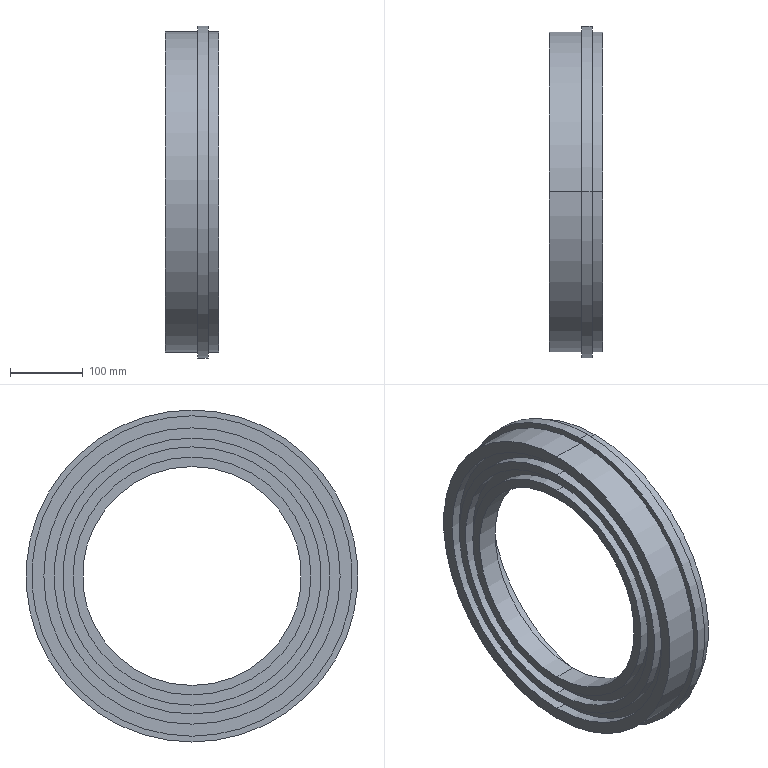Part | SolidWorks | features Revolution 1 | 1 solid | 27 faces | box 74 x 455 x 455 mm | volume 3257613 mm3 | cylinder 18 | plane 9 | commonest cylinder face diameters 439 x4 300 x2 326 x2 354 x2 378 x2 400 x2
STEP:
#1=CARTESIAN_POINT('',(74.,0.,-200.));
#2=VERTEX_POINT('',#1);
#3=CARTESIAN_POINT('',(74.,0.,200.));
#4=VERTEX_POINT('',#3);
#5=CARTESIAN_POINT('',(74.,0.,0.));
#6=DIRECTION('',(-1.,0.,0.));
#7=DIRECTION('',(0.,0.,1.));
#8=AXIS2_PLACEMENT_3D('',#5,#6,#7);
#9=CIRCLE('',#8,200.);
#10=EDGE_CURVE('',#2,#4,#9,.T.);
#11=ORIENTED_EDGE('',*,*,#10,.F.);
#12=CARTESIAN_POINT('',(30.,0.,-200.));
#13=VERTEX_POINT('',#12);
#14=CARTESIAN_POINT('',(0.,0.,-200.));
#15=DIRECTION('',(-1.,0.,0.));
#16=VECTOR('',#15,1000.);
#17=LINE('',#14,#16);
#18=EDGE_CURVE('',#2,#13,#17,.T.);
#19=ORIENTED_EDGE('',*,*,#18,.T.);
#20=CARTESIAN_POINT('',(30.,0.,200.));
#21=VERTEX_POINT('',#20);
#22=CARTESIAN_POINT('',(30.,0.,0.));
#23=DIRECTION('',(-1.,0.,0.));
#24=DIRECTION('',(0.,0.,1.));
#25=AXIS2_PLACEMENT_3D('',#22,#23,#24);
#26=CIRCLE('',#25,200.);
#27=EDGE_CURVE('',#13,#21,#26,.T.);
#28=ORIENTED_EDGE('',*,*,#27,.T.);
#29=CARTESIAN_POINT('',(0.,0.,200.));
#30=DIRECTION('',(-1.,0.,0.));
#31=VECTOR('',#30,1000.);
#32=LINE('',#29,#31);
#33=EDGE_CURVE('',#4,#21,#32,.T.);
#34=ORIENTED_EDGE('',*,*,#33,.F.);
#35=EDGE_LOOP('',(#11,#19,#28,#34));
#36=FACE_OUTER_BOUND('',#35,.T.);
#37=CARTESIAN_POINT('',(0.,0.,0.));
#38=DIRECTION('',(-1.,0.,0.));
#39=DIRECTION('',(0.,0.,1.));
#40=AXIS2_PLACEMENT_3D('',#37,#38,#39);
#41=CYLINDRICAL_SURFACE('',#40,200.);
#42=ADVANCED_FACE('',(#36),#41,.F.);
#43=CARTESIAN_POINT('',(74.,0.,219.5));
#44=VERTEX_POINT('',#43);
#45=CARTESIAN_POINT('',(74.,0.,-219.5));
#46=VERTEX_POINT('',#45);
#47=CARTESIAN_POINT('',(74.,0.,0.));
#48=DIRECTION('',(-1.,0.,0.));
#49=DIRECTION('',(0.,0.,1.));
#50=AXIS2_PLACEMENT_3D('',#47,#48,#49);
#51=CIRCLE('',#50,219.5);
#52=EDGE_CURVE('',#44,#46,#51,.T.);
#53=ORIENTED_EDGE('',*,*,#52,.T.);
#54=CARTESIAN_POINT('',(59.,0.,-219.5));
#55=VERTEX_POINT('',#54);
#56=CARTESIAN_POINT('',(0.,0.,-219.5));
#57=DIRECTION('',(-1.,0.,0.));
#58=VECTOR('',#57,1000.);
#59=LINE('',#56,#58);
#60=EDGE_CURVE('',#46,#55,#59,.T.);
#61=ORIENTED_EDGE('',*,*,#60,.T.);
#62=CARTESIAN_POINT('',(59.,0.,219.5));
#63=VERTEX_POINT('',#62);
#64=CARTESIAN_POINT('',(59.,0.,0.));
#65=DIRECTION('',(-1.,0.,0.));
#66=DIRECTION('',(0.,0.,1.));
#67=AXIS2_PLACEMENT_3D('',#64,#65,#66);
#68=CIRCLE('',#67,219.5);
#69=EDGE_CURVE('',#63,#55,#68,.T.);
#70=ORIENTED_EDGE('',*,*,#69,.F.);
#71=CARTESIAN_POINT('',(0.,0.,219.5));
#72=DIRECTION('',(-1.,0.,0.));
#73=VECTOR('',#72,1000.);
#74=LINE('',#71,#73);
#75=EDGE_CURVE('',#44,#63,#74,.T.);
#76=ORIENTED_EDGE('',*,*,#75,.F.);
#77=EDGE_LOOP('',(#53,#61,#70,#76));
#78=FACE_OUTER_BOUND('',#77,.T.);
#79=CARTESIAN_POINT('',(0.,0.,0.));
#80=DIRECTION('',(-1.,0.,0.));
#81=DIRECTION('',(0.,0.,1.));
#82=AXIS2_PLACEMENT_3D('',#79,#80,#81);
#83=CYLINDRICAL_SURFACE('',#82,219.5);
#84=ADVANCED_FACE('',(#78),#83,.T.);
#85=CARTESIAN_POINT('',(59.,0.,227.5));
#86=VERTEX_POINT('',#85);
#87=CARTESIAN_POINT('',(59.,0.,-227.5));
#88=VERTEX_POINT('',#87);
#89=CARTESIAN_POINT('',(59.,0.,0.));
#90=DIRECTION('',(-1.,0.,0.));
#91=DIRECTION('',(0.,0.,1.));
#92=AXIS2_PLACEMENT_3D('',#89,#90,#91);
#93=CIRCLE('',#92,227.5);
#94=EDGE_CURVE('',#86,#88,#93,.T.);
#95=ORIENTED_EDGE('',*,*,#94,.T.);
#96=CARTESIAN_POINT('',(45.,0.,-227.5));
#97=VERTEX_POINT('',#96);
#98=CARTESIAN_POINT('',(0.,0.,-227.5));
#99=DIRECTION('',(-1.,0.,0.));
#100=VECTOR('',#99,1000.);
#101=LINE('',#98,#100);
#102=EDGE_CURVE('',#88,#97,#101,.T.);
#103=ORIENTED_EDGE('',*,*,#102,.T.);
#104=CARTESIAN_POINT('',(45.,0.,227.5));
#105=VERTEX_POINT('',#104);
#106=CARTESIAN_POINT('',(45.,0.,0.));
#107=DIRECTION('',(-1.,0.,0.));
#108=DIRECTION('',(0.,0.,1.));
#109=AXIS2_PLACEMENT_3D('',#106,#107,#108);
#110=CIRCLE('',#109,227.5);
#111=EDGE_CURVE('',#105,#97,#110,.T.);
#112=ORIENTED_EDGE('',*,*,#111,.F.);
#113=CARTESIAN_POINT('',(0.,0.,227.5));
#114=DIRECTION('',(-1.,0.,0.));
#115=VECTOR('',#114,1000.);
#116=LINE('',#113,#115);
#117=EDGE_CURVE('',#86,#105,#116,.T.);
#118=ORIENTED_EDGE('',*,*,#117,.F.);
#119=EDGE_LOOP('',(#95,#103,#112,#118));
#120=FACE_OUTER_BOUND('',#119,.T.);
#121=CARTESIAN_POINT('',(0.,0.,0.));
#122=DIRECTION('',(-1.,0.,0.));
#123=DIRECTION('',(0.,0.,1.));
#124=AXIS2_PLACEMENT_3D('',#121,#122,#123);
#125=CYLINDRICAL_SURFACE('',#124,227.5);
#126=ADVANCED_FACE('',(#120),#125,.T.);
#127=CARTESIAN_POINT('',(45.,0.,219.5));
#128=VERTEX_POINT('',#127);
#129=CARTESIAN_POINT('',(45.,0.,-219.5));
#130=VERTEX_POINT('',#129);
#131=CARTESIAN_POINT('',(45.,0.,0.));
#132=DIRECTION('',(-1.,0.,0.));
#133=DIRECTION('',(0.,0.,1.));
#134=AXIS2_PLACEMENT_3D('',#131,#132,#133);
#135=CIRCLE('',#134,219.5);
#136=EDGE_CURVE('',#128,#130,#135,.T.);
#137=ORIENTED_EDGE('',*,*,#136,.T.);
#138=CARTESIAN_POINT('',(0.,0.,-219.5));
#139=VERTEX_POINT('',#138);
#140=CARTESIAN_POINT('',(0.,0.,-219.5));
#141=DIRECTION('',(-1.,0.,0.));
#142=VECTOR('',#141,1000.);
#143=LINE('',#140,#142);
#144=EDGE_CURVE('',#130,#139,#143,.T.);
#145=ORIENTED_EDGE('',*,*,#144,.T.);
#146=CARTESIAN_POINT('',(0.,0.,219.5));
#147=VERTEX_POINT('',#146);
#148=CARTESIAN_POINT('',(0.,0.,0.));
#149=DIRECTION('',(-1.,0.,0.));
#150=DIRECTION('',(0.,0.,1.));
#151=AXIS2_PLACEMENT_3D('',#148,#149,#150);
#152=CIRCLE('',#151,219.5);
#153=EDGE_CURVE('',#147,#139,#152,.T.);
#154=ORIENTED_EDGE('',*,*,#153,.F.);
#155=CARTESIAN_POINT('',(0.,0.,219.5));
#156=DIRECTION('',(-1.,0.,0.));
#157=VECTOR('',#156,1000.);
#158=LINE('',#155,#157);
#159=EDGE_CURVE('',#128,#147,#158,.T.);
#160=ORIENTED_EDGE('',*,*,#159,.F.);
#161=EDGE_LOOP('',(#137,#145,#154,#160));
#162=FACE_OUTER_BOUND('',#161,.T.);
#163=CARTESIAN_POINT('',(0.,0.,0.));
#164=DIRECTION('',(-1.,0.,0.));
#165=DIRECTION('',(0.,0.,1.));
#166=AXIS2_PLACEMENT_3D('',#163,#164,#165);
#167=CYLINDRICAL_SURFACE('',#166,219.5);
#168=ADVANCED_FACE('',(#162),#167,.T.);
#169=CARTESIAN_POINT('',(14.,0.,-203.));
#170=VERTEX_POINT('',#169);
#171=CARTESIAN_POINT('',(14.,0.,203.));
#172=VERTEX_POINT('',#171);
#173=CARTESIAN_POINT('',(14.,0.,0.));
#174=DIRECTION('',(-1.,0.,0.));
#175=DIRECTION('',(0.,0.,1.));
#176=AXIS2_PLACEMENT_3D('',#173,#174,#175);
#177=CIRCLE('',#176,203.);
#178=EDGE_CURVE('',#170,#172,#177,.T.);
#179=ORIENTED_EDGE('',*,*,#178,.F.);
#180=CARTESIAN_POINT('',(0.,0.,-203.));
#181=VERTEX_POINT('',#180);
#182=CARTESIAN_POINT('',(0.,0.,-203.));
#183=DIRECTION('',(-1.,0.,0.));
#184=VECTOR('',#183,1000.);
#185=LINE('',#182,#184);
#186=EDGE_CURVE('',#170,#181,#185,.T.);
#187=ORIENTED_EDGE('',*,*,#186,.T.);
#188=CARTESIAN_POINT('',(0.,0.,203.));
#189=VERTEX_POINT('',#188);
#190=CARTESIAN_POINT('',(0.,0.,0.));
#191=DIRECTION('',(-1.,0.,0.));
#192=DIRECTION('',(0.,0.,1.));
#193=AXIS2_PLACEMENT_3D('',#190,#191,#192);
#194=CIRCLE('',#193,203.);
#195=EDGE_CURVE('',#181,#189,#194,.T.);
#196=ORIENTED_EDGE('',*,*,#195,.T.);
#197=CARTESIAN_POINT('',(0.,0.,203.));
#198=DIRECTION('',(-1.,0.,0.));
#199=VECTOR('',#198,1000.);
#200=LINE('',#197,#199);
#201=EDGE_CURVE('',#172,#189,#200,.T.);
#202=ORIENTED_EDGE('',*,*,#201,.F.);
#203=EDGE_LOOP('',(#179,#187,#196,#202));
#204=FACE_OUTER_BOUND('',#203,.T.);
#205=CARTESIAN_POINT('',(0.,0.,0.));
#206=DIRECTION('',(-1.,0.,0.));
#207=DIRECTION('',(0.,0.,1.));
#208=AXIS2_PLACEMENT_3D('',#205,#206,#207);
#209=CYLINDRICAL_SURFACE('',#208,203.);
#210=ADVANCED_FACE('',(#204),#209,.F.);
#211=CARTESIAN_POINT('',(14.,0.,189.));
#212=VERTEX_POINT('',#211);
#213=CARTESIAN_POINT('',(14.,0.,-189.));
#214=VERTEX_POINT('',#213);
#215=CARTESIAN_POINT('',(14.,0.,0.));
#216=DIRECTION('',(-1.,0.,0.));
#217=DIRECTION('',(0.,0.,1.));
#218=AXIS2_PLACEMENT_3D('',#215,#216,#217);
#219=CIRCLE('',#218,189.);
#220=EDGE_CURVE('',#212,#214,#219,.T.);
#221=ORIENTED_EDGE('',*,*,#220,.T.);
#222=CARTESIAN_POINT('',(0.,0.,-189.));
#223=VERTEX_POINT('',#222);
#224=CARTESIAN_POINT('',(0.,0.,-189.));
#225=DIRECTION('',(-1.,0.,0.));
#226=VECTOR('',#225,1000.);
#227=LINE('',#224,#226);
#228=EDGE_CURVE('',#214,#223,#227,.T.);
#229=ORIENTED_EDGE('',*,*,#228,.T.);
#230=CARTESIAN_POINT('',(0.,0.,189.));
#231=VERTEX_POINT('',#230);
#232=CARTESIAN_POINT('',(0.,0.,0.));
#233=DIRECTION('',(-1.,0.,0.));
#234=DIRECTION('',(0.,0.,1.));
#235=AXIS2_PLACEMENT_3D('',#232,#233,#234);
#236=CIRCLE('',#235,189.);
#237=EDGE_CURVE('',#231,#223,#236,.T.);
#238=ORIENTED_EDGE('',*,*,#237,.F.);
#239=CARTESIAN_POINT('',(0.,0.,189.));
#240=DIRECTION('',(-1.,0.,0.));
#241=VECTOR('',#240,1000.);
#242=LINE('',#239,#241);
#243=EDGE_CURVE('',#212,#231,#242,.T.);
#244=ORIENTED_EDGE('',*,*,#243,.F.);
#245=EDGE_LOOP('',(#221,#229,#238,#244));
#246=FACE_OUTER_BOUND('',#245,.T.);
#247=CARTESIAN_POINT('',(0.,0.,0.));
#248=DIRECTION('',(-1.,0.,0.));
#249=DIRECTION('',(0.,0.,1.));
#250=AXIS2_PLACEMENT_3D('',#247,#248,#249);
#251=CYLINDRICAL_SURFACE('',#250,189.);
#252=ADVANCED_FACE('',(#246),#251,.T.);
#253=CARTESIAN_POINT('',(14.,0.,-177.));
#254=VERTEX_POINT('',#253);
#255=CARTESIAN_POINT('',(14.,0.,177.));
#256=VERTEX_POINT('',#255);
#257=CARTESIAN_POINT('',(14.,0.,0.));
#258=DIRECTION('',(-1.,0.,0.));
#259=DIRECTION('',(0.,0.,1.));
#260=AXIS2_PLACEMENT_3D('',#257,#258,#259);
#261=CIRCLE('',#260,177.);
#262=EDGE_CURVE('',#254,#256,#261,.T.);
#263=ORIENTED_EDGE('',*,*,#262,.F.);
#264=CARTESIAN_POINT('',(0.,0.,-177.));
#265=VERTEX_POINT('',#264);
#266=CARTESIAN_POINT('',(0.,0.,-177.));
#267=DIRECTION('',(-1.,0.,0.));
#268=VECTOR('',#267,1000.);
#269=LINE('',#266,#268);
#270=EDGE_CURVE('',#254,#265,#269,.T.);
#271=ORIENTED_EDGE('',*,*,#270,.T.);
#272=CARTESIAN_POINT('',(0.,0.,177.));
#273=VERTEX_POINT('',#272);
#274=CARTESIAN_POINT('',(0.,0.,0.));
#275=DIRECTION('',(-1.,0.,0.));
#276=DIRECTION('',(0.,0.,1.));
#277=AXIS2_PLACEMENT_3D('',#274,#275,#276);
#278=CIRCLE('',#277,177.);
#279=EDGE_CURVE('',#265,#273,#278,.T.);
#280=ORIENTED_EDGE('',*,*,#279,.T.);
#281=CARTESIAN_POINT('',(0.,0.,177.));
#282=DIRECTION('',(-1.,0.,0.));
#283=VECTOR('',#282,1000.);
#284=LINE('',#281,#283);
#285=EDGE_CURVE('',#256,#273,#284,.T.);
#286=ORIENTED_EDGE('',*,*,#285,.F.);
#287=EDGE_LOOP('',(#263,#271,#280,#286));
#288=FACE_OUTER_BOUND('',#287,.T.);
#289=CARTESIAN_POINT('',(0.,0.,0.));
#290=DIRECTION('',(-1.,0.,0.));
#291=DIRECTION('',(0.,0.,1.));
#292=AXIS2_PLACEMENT_3D('',#289,#290,#291);
#293=CYLINDRICAL_SURFACE('',#292,177.);
#294=ADVANCED_FACE('',(#288),#293,.F.);
#295=CARTESIAN_POINT('',(14.,0.,163.));
#296=VERTEX_POINT('',#295);
#297=CARTESIAN_POINT('',(14.,0.,-163.));
#298=VERTEX_POINT('',#297);
#299=CARTESIAN_POINT('',(14.,0.,0.));
#300=DIRECTION('',(-1.,0.,0.));
#301=DIRECTION('',(0.,0.,1.));
#302=AXIS2_PLACEMENT_3D('',#299,#300,#301);
#303=CIRCLE('',#302,163.);
#304=EDGE_CURVE('',#296,#298,#303,.T.);
#305=ORIENTED_EDGE('',*,*,#304,.T.);
#306=CARTESIAN_POINT('',(0.,0.,-163.));
#307=VERTEX_POINT('',#306);
#308=CARTESIAN_POINT('',(0.,0.,-163.));
#309=DIRECTION('',(-1.,0.,0.));
#310=VECTOR('',#309,1000.);
#311=LINE('',#308,#310);
#312=EDGE_CURVE('',#298,#307,#311,.T.);
#313=ORIENTED_EDGE('',*,*,#312,.T.);
#314=CARTESIAN_POINT('',(0.,0.,163.));
#315=VERTEX_POINT('',#314);
#316=CARTESIAN_POINT('',(0.,0.,0.));
#317=DIRECTION('',(-1.,0.,0.));
#318=DIRECTION('',(0.,0.,1.));
#319=AXIS2_PLACEMENT_3D('',#316,#317,#318);
#320=CIRCLE('',#319,163.);
#321=EDGE_CURVE('',#315,#307,#320,.T.);
#322=ORIENTED_EDGE('',*,*,#321,.F.);
#323=CARTESIAN_POINT('',(0.,0.,163.));
#324=DIRECTION('',(-1.,0.,0.));
#325=VECTOR('',#324,1000.);
#326=LINE('',#323,#325);
#327=EDGE_CURVE('',#296,#315,#326,.T.);
#328=ORIENTED_EDGE('',*,*,#327,.F.);
#329=EDGE_LOOP('',(#305,#313,#322,#328));
#330=FACE_OUTER_BOUND('',#329,.T.);
#331=CARTESIAN_POINT('',(0.,0.,0.));
#332=DIRECTION('',(-1.,0.,0.));
#333=DIRECTION('',(0.,0.,1.));
#334=AXIS2_PLACEMENT_3D('',#331,#332,#333);
#335=CYLINDRICAL_SURFACE('',#334,163.);
#336=ADVANCED_FACE('',(#330),#335,.T.);
#337=CARTESIAN_POINT('',(30.,0.,-150.));
#338=VERTEX_POINT('',#337);
#339=CARTESIAN_POINT('',(30.,0.,150.));
#340=VERTEX_POINT('',#339);
#341=CARTESIAN_POINT('',(30.,0.,0.));
#342=DIRECTION('',(-1.,0.,0.));
#343=DIRECTION('',(0.,0.,1.));
#344=AXIS2_PLACEMENT_3D('',#341,#342,#343);
#345=CIRCLE('',#344,150.);
#346=EDGE_CURVE('',#338,#340,#345,.T.);
#347=ORIENTED_EDGE('',*,*,#346,.F.);
#348=CARTESIAN_POINT('',(0.,0.,-150.));
#349=VERTEX_POINT('',#348);
#350=CARTESIAN_POINT('',(0.,0.,-150.));
#351=DIRECTION('',(-1.,0.,0.));
#352=VECTOR('',#351,1000.);
#353=LINE('',#350,#352);
#354=EDGE_CURVE('',#338,#349,#353,.T.);
#355=ORIENTED_EDGE('',*,*,#354,.T.);
#356=CARTESIAN_POINT('',(0.,0.,150.));
#357=VERTEX_POINT('',#356);
#358=CARTESIAN_POINT('',(0.,0.,0.));
#359=DIRECTION('',(-1.,0.,0.));
#360=DIRECTION('',(0.,0.,1.));
#361=AXIS2_PLACEMENT_3D('',#358,#359,#360);
#362=CIRCLE('',#361,150.);
#363=EDGE_CURVE('',#349,#357,#362,.T.);
#364=ORIENTED_EDGE('',*,*,#363,.T.);
#365=CARTESIAN_POINT('',(0.,0.,150.));
#366=DIRECTION('',(-1.,0.,0.));
#367=VECTOR('',#366,1000.);
#368=LINE('',#365,#367);
#369=EDGE_CURVE('',#340,#357,#368,.T.);
#370=ORIENTED_EDGE('',*,*,#369,.F.);
#371=EDGE_LOOP('',(#347,#355,#364,#370));
#372=FACE_OUTER_BOUND('',#371,.T.);
#373=CARTESIAN_POINT('',(0.,0.,0.));
#374=DIRECTION('',(-1.,0.,0.));
#375=DIRECTION('',(0.,0.,1.));
#376=AXIS2_PLACEMENT_3D('',#373,#374,#375);
#377=CYLINDRICAL_SURFACE('',#376,150.);
#378=ADVANCED_FACE('',(#372),#377,.F.);
#379=ORIENTED_EDGE('',*,*,#354,.F.);
#380=CARTESIAN_POINT('',(30.,0.,0.));
#381=DIRECTION('',(-1.,0.,0.));
#382=DIRECTION('',(0.,0.,1.));
#383=AXIS2_PLACEMENT_3D('',#380,#381,#382);
#384=CIRCLE('',#383,150.);
#385=EDGE_CURVE('',#340,#338,#384,.T.);
#386=ORIENTED_EDGE('',*,*,#385,.F.);
#387=ORIENTED_EDGE('',*,*,#369,.T.);
#388=CARTESIAN_POINT('',(0.,0.,0.));
#389=DIRECTION('',(-1.,0.,0.));
#390=DIRECTION('',(0.,0.,1.));
#391=AXIS2_PLACEMENT_3D('',#388,#389,#390);
#392=CIRCLE('',#391,150.);
#393=EDGE_CURVE('',#357,#349,#392,.T.);
#394=ORIENTED_EDGE('',*,*,#393,.T.);
#395=EDGE_LOOP('',(#379,#386,#387,#394));
#396=FACE_OUTER_BOUND('',#395,.T.);
#397=CARTESIAN_POINT('',(0.,0.,0.));
#398=DIRECTION('',(-1.,0.,0.));
#399=DIRECTION('',(0.,0.,1.));
#400=AXIS2_PLACEMENT_3D('',#397,#398,#399);
#401=CYLINDRICAL_SURFACE('',#400,150.);
#402=ADVANCED_FACE('',(#396),#401,.F.);
#403=ORIENTED_EDGE('',*,*,#393,.F.);
#404=ORIENTED_EDGE('',*,*,#363,.F.);
#405=EDGE_LOOP('',(#403,#404));
#406=FACE_BOUND('',#405,.T.);
#407=ORIENTED_EDGE('',*,*,#321,.T.);
#408=CARTESIAN_POINT('',(0.,0.,0.));
#409=DIRECTION('',(-1.,0.,0.));
#410=DIRECTION('',(0.,0.,1.));
#411=AXIS2_PLACEMENT_3D('',#408,#409,#410);
#412=CIRCLE('',#411,163.);
#413=EDGE_CURVE('',#307,#315,#412,.T.);
#414=ORIENTED_EDGE('',*,*,#413,.T.);
#415=EDGE_LOOP('',(#407,#414));
#416=FACE_OUTER_BOUND('',#415,.T.);
#417=CARTESIAN_POINT('',(0.,0.,-150.));
#418=DIRECTION('',(1.,0.,0.));
#419=DIRECTION('',(0.,0.,-1.));
#420=AXIS2_PLACEMENT_3D('',#417,#418,#419);
#421=PLANE('',#420);
#422=ADVANCED_FACE('',(#406,#416),#421,.F.);
#423=ORIENTED_EDGE('',*,*,#312,.F.);
#424=CARTESIAN_POINT('',(14.,0.,0.));
#425=DIRECTION('',(-1.,0.,0.));
#426=DIRECTION('',(0.,0.,1.));
#427=AXIS2_PLACEMENT_3D('',#424,#425,#426);
#428=CIRCLE('',#427,163.);
#429=EDGE_CURVE('',#298,#296,#428,.T.);
#430=ORIENTED_EDGE('',*,*,#429,.T.);
#431=ORIENTED_EDGE('',*,*,#327,.T.);
#432=ORIENTED_EDGE('',*,*,#413,.F.);
#433=EDGE_LOOP('',(#423,#430,#431,#432));
#434=FACE_OUTER_BOUND('',#433,.T.);
#435=CARTESIAN_POINT('',(0.,0.,0.));
#436=DIRECTION('',(-1.,0.,0.));
#437=DIRECTION('',(0.,0.,1.));
#438=AXIS2_PLACEMENT_3D('',#435,#436,#437);
#439=CYLINDRICAL_SURFACE('',#438,163.);
#440=ADVANCED_FACE('',(#434),#439,.T.);
#441=ORIENTED_EDGE('',*,*,#304,.F.);
#442=ORIENTED_EDGE('',*,*,#429,.F.);
#443=EDGE_LOOP('',(#441,#442));
#444=FACE_BOUND('',#443,.T.);
#445=CARTESIAN_POINT('',(14.,0.,0.));
#446=DIRECTION('',(-1.,0.,0.));
#447=DIRECTION('',(0.,0.,1.));
#448=AXIS2_PLACEMENT_3D('',#445,#446,#447);
#449=CIRCLE('',#448,177.);
#450=EDGE_CURVE('',#256,#254,#449,.T.);
#451=ORIENTED_EDGE('',*,*,#450,.T.);
#452=ORIENTED_EDGE('',*,*,#262,.T.);
#453=EDGE_LOOP('',(#451,#452));
#454=FACE_OUTER_BOUND('',#453,.T.);
#455=CARTESIAN_POINT('',(14.,0.,-177.));
#456=DIRECTION('',(1.,0.,0.));
#457=DIRECTION('',(0.,0.,-1.));
#458=AXIS2_PLACEMENT_3D('',#455,#456,#457);
#459=PLANE('',#458);
#460=ADVANCED_FACE('',(#444,#454),#459,.F.);
#461=ORIENTED_EDGE('',*,*,#270,.F.);
#462=ORIENTED_EDGE('',*,*,#450,.F.);
#463=ORIENTED_EDGE('',*,*,#285,.T.);
#464=CARTESIAN_POINT('',(0.,0.,0.));
#465=DIRECTION('',(-1.,0.,0.));
#466=DIRECTION('',(0.,0.,1.));
#467=AXIS2_PLACEMENT_3D('',#464,#465,#466);
#468=CIRCLE('',#467,177.);
#469=EDGE_CURVE('',#273,#265,#468,.T.);
#470=ORIENTED_EDGE('',*,*,#469,.T.);
#471=EDGE_LOOP('',(#461,#462,#463,#470));
#472=FACE_OUTER_BOUND('',#471,.T.);
#473=CARTESIAN_POINT('',(0.,0.,0.));
#474=DIRECTION('',(-1.,0.,0.));
#475=DIRECTION('',(0.,0.,1.));
#476=AXIS2_PLACEMENT_3D('',#473,#474,#475);
#477=CYLINDRICAL_SURFACE('',#476,177.);
#478=ADVANCED_FACE('',(#472),#477,.F.);
#479=ORIENTED_EDGE('',*,*,#469,.F.);
#480=ORIENTED_EDGE('',*,*,#279,.F.);
#481=EDGE_LOOP('',(#479,#480));
#482=FACE_BOUND('',#481,.T.);
#483=ORIENTED_EDGE('',*,*,#237,.T.);
#484=CARTESIAN_POINT('',(0.,0.,0.));
#485=DIRECTION('',(-1.,0.,0.));
#486=DIRECTION('',(0.,0.,1.));
#487=AXIS2_PLACEMENT_3D('',#484,#485,#486);
#488=CIRCLE('',#487,189.);
#489=EDGE_CURVE('',#223,#231,#488,.T.);
#490=ORIENTED_EDGE('',*,*,#489,.T.);
#491=EDGE_LOOP('',(#483,#490));
#492=FACE_OUTER_BOUND('',#491,.T.);
#493=CARTESIAN_POINT('',(0.,0.,-177.));
#494=DIRECTION('',(1.,0.,0.));
#495=DIRECTION('',(0.,0.,-1.));
#496=AXIS2_PLACEMENT_3D('',#493,#494,#495);
#497=PLANE('',#496);
#498=ADVANCED_FACE('',(#482,#492),#497,.F.);
#499=ORIENTED_EDGE('',*,*,#228,.F.);
#500=CARTESIAN_POINT('',(14.,0.,0.));
#501=DIRECTION('',(-1.,0.,0.));
#502=DIRECTION('',(0.,0.,1.));
#503=AXIS2_PLACEMENT_3D('',#500,#501,#502);
#504=CIRCLE('',#503,189.);
#505=EDGE_CURVE('',#214,#212,#504,.T.);
#506=ORIENTED_EDGE('',*,*,#505,.T.);
#507=ORIENTED_EDGE('',*,*,#243,.T.);
#508=ORIENTED_EDGE('',*,*,#489,.F.);
#509=EDGE_LOOP('',(#499,#506,#507,#508));
#510=FACE_OUTER_BOUND('',#509,.T.);
#511=CARTESIAN_POINT('',(0.,0.,0.));
#512=DIRECTION('',(-1.,0.,0.));
#513=DIRECTION('',(0.,0.,1.));
#514=AXIS2_PLACEMENT_3D('',#511,#512,#513);
#515=CYLINDRICAL_SURFACE('',#514,189.);
#516=ADVANCED_FACE('',(#510),#515,.T.);
#517=ORIENTED_EDGE('',*,*,#220,.F.);
#518=ORIENTED_EDGE('',*,*,#505,.F.);
#519=EDGE_LOOP('',(#517,#518));
#520=FACE_BOUND('',#519,.T.);
#521=CARTESIAN_POINT('',(14.,0.,0.));
#522=DIRECTION('',(-1.,0.,0.));
#523=DIRECTION('',(0.,0.,1.));
#524=AXIS2_PLACEMENT_3D('',#521,#522,#523);
#525=CIRCLE('',#524,203.);
#526=EDGE_CURVE('',#172,#170,#525,.T.);
#527=ORIENTED_EDGE('',*,*,#526,.T.);
#528=ORIENTED_EDGE('',*,*,#178,.T.);
#529=EDGE_LOOP('',(#527,#528));
#530=FACE_OUTER_BOUND('',#529,.T.);
#531=CARTESIAN_POINT('',(14.,0.,-203.));
#532=DIRECTION('',(1.,0.,0.));
#533=DIRECTION('',(0.,0.,-1.));
#534=AXIS2_PLACEMENT_3D('',#531,#532,#533);
#535=PLANE('',#534);
#536=ADVANCED_FACE('',(#520,#530),#535,.F.);
#537=ORIENTED_EDGE('',*,*,#186,.F.);
#538=ORIENTED_EDGE('',*,*,#526,.F.);
#539=ORIENTED_EDGE('',*,*,#201,.T.);
#540=CARTESIAN_POINT('',(0.,0.,0.));
#541=DIRECTION('',(-1.,0.,0.));
#542=DIRECTION('',(0.,0.,1.));
#543=AXIS2_PLACEMENT_3D('',#540,#541,#542);
#544=CIRCLE('',#543,203.);
#545=EDGE_CURVE('',#189,#181,#544,.T.);
#546=ORIENTED_EDGE('',*,*,#545,.T.);
#547=EDGE_LOOP('',(#537,#538,#539,#546));
#548=FACE_OUTER_BOUND('',#547,.T.);
#549=CARTESIAN_POINT('',(0.,0.,0.));
#550=DIRECTION('',(-1.,0.,0.));
#551=DIRECTION('',(0.,0.,1.));
#552=AXIS2_PLACEMENT_3D('',#549,#550,#551);
#553=CYLINDRICAL_SURFACE('',#552,203.);
#554=ADVANCED_FACE('',(#548),#553,.F.);
#555=ORIENTED_EDGE('',*,*,#545,.F.);
#556=ORIENTED_EDGE('',*,*,#195,.F.);
#557=EDGE_LOOP('',(#555,#556));
#558=FACE_BOUND('',#557,.T.);
#559=ORIENTED_EDGE('',*,*,#153,.T.);
#560=CARTESIAN_POINT('',(0.,0.,0.));
#561=DIRECTION('',(-1.,0.,0.));
#562=DIRECTION('',(0.,0.,1.));
#563=AXIS2_PLACEMENT_3D('',#560,#561,#562);
#564=CIRCLE('',#563,219.5);
#565=EDGE_CURVE('',#139,#147,#564,.T.);
#566=ORIENTED_EDGE('',*,*,#565,.T.);
#567=EDGE_LOOP('',(#559,#566));
#568=FACE_OUTER_BOUND('',#567,.T.);
#569=CARTESIAN_POINT('',(0.,0.,-203.));
#570=DIRECTION('',(1.,0.,0.));
#571=DIRECTION('',(0.,0.,-1.));
#572=AXIS2_PLACEMENT_3D('',#569,#570,#571);
#573=PLANE('',#572);
#574=ADVANCED_FACE('',(#558,#568),#573,.F.);
#575=ORIENTED_EDGE('',*,*,#144,.F.);
#576=CARTESIAN_POINT('',(45.,0.,0.));
#577=DIRECTION('',(-1.,0.,0.));
#578=DIRECTION('',(0.,0.,1.));
#579=AXIS2_PLACEMENT_3D('',#576,#577,#578);
#580=CIRCLE('',#579,219.5);
#581=EDGE_CURVE('',#130,#128,#580,.T.);
#582=ORIENTED_EDGE('',*,*,#581,.T.);
#583=ORIENTED_EDGE('',*,*,#159,.T.);
#584=ORIENTED_EDGE('',*,*,#565,.F.);
#585=EDGE_LOOP('',(#575,#582,#583,#584));
#586=FACE_OUTER_BOUND('',#585,.T.);
#587=CARTESIAN_POINT('',(0.,0.,0.));
#588=DIRECTION('',(-1.,0.,0.));
#589=DIRECTION('',(0.,0.,1.));
#590=AXIS2_PLACEMENT_3D('',#587,#588,#589);
#591=CYLINDRICAL_SURFACE('',#590,219.5);
#592=ADVANCED_FACE('',(#586),#591,.T.);
#593=ORIENTED_EDGE('',*,*,#136,.F.);
#594=ORIENTED_EDGE('',*,*,#581,.F.);
#595=EDGE_LOOP('',(#593,#594));
#596=FACE_BOUND('',#595,.T.);
#597=ORIENTED_EDGE('',*,*,#111,.T.);
#598=CARTESIAN_POINT('',(45.,0.,0.));
#599=DIRECTION('',(-1.,0.,0.));
#600=DIRECTION('',(0.,0.,1.));
#601=AXIS2_PLACEMENT_3D('',#598,#599,#600);
#602=CIRCLE('',#601,227.5);
#603=EDGE_CURVE('',#97,#105,#602,.T.);
#604=ORIENTED_EDGE('',*,*,#603,.T.);
#605=EDGE_LOOP('',(#597,#604));
#606=FACE_OUTER_BOUND('',#605,.T.);
#607=CARTESIAN_POINT('',(45.,0.,-219.5));
#608=DIRECTION('',(1.,0.,0.));
#609=DIRECTION('',(0.,0.,-1.));
#610=AXIS2_PLACEMENT_3D('',#607,#608,#609);
#611=PLANE('',#610);
#612=ADVANCED_FACE('',(#596,#606),#611,.F.);
#613=ORIENTED_EDGE('',*,*,#102,.F.);
#614=CARTESIAN_POINT('',(59.,0.,0.));
#615=DIRECTION('',(-1.,0.,0.));
#616=DIRECTION('',(0.,0.,1.));
#617=AXIS2_PLACEMENT_3D('',#614,#615,#616);
#618=CIRCLE('',#617,227.5);
#619=EDGE_CURVE('',#88,#86,#618,.T.);
#620=ORIENTED_EDGE('',*,*,#619,.T.);
#621=ORIENTED_EDGE('',*,*,#117,.T.);
#622=ORIENTED_EDGE('',*,*,#603,.F.);
#623=EDGE_LOOP('',(#613,#620,#621,#622));
#624=FACE_OUTER_BOUND('',#623,.T.);
#625=CARTESIAN_POINT('',(0.,0.,0.));
#626=DIRECTION('',(-1.,0.,0.));
#627=DIRECTION('',(0.,0.,1.));
#628=AXIS2_PLACEMENT_3D('',#625,#626,#627);
#629=CYLINDRICAL_SURFACE('',#628,227.5);
#630=ADVANCED_FACE('',(#624),#629,.T.);
#631=ORIENTED_EDGE('',*,*,#94,.F.);
#632=ORIENTED_EDGE('',*,*,#619,.F.);
#633=EDGE_LOOP('',(#631,#632));
#634=FACE_OUTER_BOUND('',#633,.T.);
#635=ORIENTED_EDGE('',*,*,#69,.T.);
#636=CARTESIAN_POINT('',(59.,0.,0.));
#637=DIRECTION('',(-1.,0.,0.));
#638=DIRECTION('',(0.,0.,1.));
#639=AXIS2_PLACEMENT_3D('',#636,#637,#638);
#640=CIRCLE('',#639,219.5);
#641=EDGE_CURVE('',#55,#63,#640,.T.);
#642=ORIENTED_EDGE('',*,*,#641,.T.);
#643=EDGE_LOOP('',(#635,#642));
#644=FACE_BOUND('',#643,.T.);
#645=CARTESIAN_POINT('',(59.,0.,-227.5));
#646=DIRECTION('',(-1.,0.,0.));
#647=DIRECTION('',(0.,0.,1.));
#648=AXIS2_PLACEMENT_3D('',#645,#646,#647);
#649=PLANE('',#648);
#650=ADVANCED_FACE('',(#634,#644),#649,.F.);
#651=ORIENTED_EDGE('',*,*,#60,.F.);
#652=CARTESIAN_POINT('',(74.,0.,0.));
#653=DIRECTION('',(-1.,0.,0.));
#654=DIRECTION('',(0.,0.,1.));
#655=AXIS2_PLACEMENT_3D('',#652,#653,#654);
#656=CIRCLE('',#655,219.5);
#657=EDGE_CURVE('',#46,#44,#656,.T.);
#658=ORIENTED_EDGE('',*,*,#657,.T.);
#659=ORIENTED_EDGE('',*,*,#75,.T.);
#660=ORIENTED_EDGE('',*,*,#641,.F.);
#661=EDGE_LOOP('',(#651,#658,#659,#660));
#662=FACE_OUTER_BOUND('',#661,.T.);
#663=CARTESIAN_POINT('',(0.,0.,0.));
#664=DIRECTION('',(-1.,0.,0.));
#665=DIRECTION('',(0.,0.,1.));
#666=AXIS2_PLACEMENT_3D('',#663,#664,#665);
#667=CYLINDRICAL_SURFACE('',#666,219.5);
#668=ADVANCED_FACE('',(#662),#667,.T.);
#669=ORIENTED_EDGE('',*,*,#52,.F.);
#670=ORIENTED_EDGE('',*,*,#657,.F.);
#671=EDGE_LOOP('',(#669,#670));
#672=FACE_OUTER_BOUND('',#671,.T.);
#673=CARTESIAN_POINT('',(74.,0.,0.));
#674=DIRECTION('',(-1.,0.,0.));
#675=DIRECTION('',(0.,0.,1.));
#676=AXIS2_PLACEMENT_3D('',#673,#674,#675);
#677=CIRCLE('',#676,200.);
#678=EDGE_CURVE('',#4,#2,#677,.T.);
#679=ORIENTED_EDGE('',*,*,#678,.T.);
#680=ORIENTED_EDGE('',*,*,#10,.T.);
#681=EDGE_LOOP('',(#679,#680));
#682=FACE_BOUND('',#681,.T.);
#683=CARTESIAN_POINT('',(74.,0.,-219.5));
#684=DIRECTION('',(-1.,0.,0.));
#685=DIRECTION('',(0.,0.,1.));
#686=AXIS2_PLACEMENT_3D('',#683,#684,#685);
#687=PLANE('',#686);
#688=ADVANCED_FACE('',(#672,#682),#687,.F.);
#689=ORIENTED_EDGE('',*,*,#18,.F.);
#690=ORIENTED_EDGE('',*,*,#678,.F.);
#691=ORIENTED_EDGE('',*,*,#33,.T.);
#692=CARTESIAN_POINT('',(30.,0.,0.));
#693=DIRECTION('',(-1.,0.,0.));
#694=DIRECTION('',(0.,0.,1.));
#695=AXIS2_PLACEMENT_3D('',#692,#693,#694);
#696=CIRCLE('',#695,200.);
#697=EDGE_CURVE('',#21,#13,#696,.T.);
#698=ORIENTED_EDGE('',*,*,#697,.T.);
#699=EDGE_LOOP('',(#689,#690,#691,#698));
#700=FACE_OUTER_BOUND('',#699,.T.);
#701=CARTESIAN_POINT('',(0.,0.,0.));
#702=DIRECTION('',(-1.,0.,0.));
#703=DIRECTION('',(0.,0.,1.));
#704=AXIS2_PLACEMENT_3D('',#701,#702,#703);
#705=CYLINDRICAL_SURFACE('',#704,200.);
#706=ADVANCED_FACE('',(#700),#705,.F.);
#707=ORIENTED_EDGE('',*,*,#697,.F.);
#708=ORIENTED_EDGE('',*,*,#27,.F.);
#709=EDGE_LOOP('',(#707,#708));
#710=FACE_OUTER_BOUND('',#709,.T.);
#711=ORIENTED_EDGE('',*,*,#385,.T.);
#712=ORIENTED_EDGE('',*,*,#346,.T.);
#713=EDGE_LOOP('',(#711,#712));
#714=FACE_BOUND('',#713,.T.);
#715=CARTESIAN_POINT('',(30.,0.,-200.));
#716=DIRECTION('',(-1.,0.,0.));
#717=DIRECTION('',(0.,0.,1.));
#718=AXIS2_PLACEMENT_3D('',#715,#716,#717);
#719=PLANE('',#718);
#720=ADVANCED_FACE('',(#710,#714),#719,.F.);
#721=CLOSED_SHELL('',(#42,#84,#126,#168,#210,#252,#294,#336,#378,#402,#422,#440,#460,#478,#498,#516,#536,#554,#574,#592,#612,#630,#650,#668,#688,#706,#720));
#722=MANIFOLD_SOLID_BREP('',#721);
#723=CARTESIAN_POINT('',(0.,0.,0.));
#724=DIRECTION('',(0.,0.,1.));
#725=DIRECTION('',(1.,0.,0.));
#726=AXIS2_PLACEMENT_3D('',#723,#724,#725);
#727=(LENGTH_UNIT()NAMED_UNIT(*)SI_UNIT(.MILLI.,.METRE.));
#728=UNCERTAINTY_MEASURE_WITH_UNIT(LENGTH_MEASURE(0.00001),#727,'','');
#729=(NAMED_UNIT(*)PLANE_ANGLE_UNIT()SI_UNIT($,.RADIAN.));
#730=(NAMED_UNIT(*)SI_UNIT($,.STERADIAN.)SOLID_ANGLE_UNIT());
#731=(GEOMETRIC_REPRESENTATION_CONTEXT(3)GLOBAL_UNCERTAINTY_ASSIGNED_CONTEXT((#728))GLOBAL_UNIT_ASSIGNED_CONTEXT((#727,#729,#730))REPRESENTATION_CONTEXT('',''));
#732=ADVANCED_BREP_SHAPE_REPRESENTATION('',(#722,#726),#731);